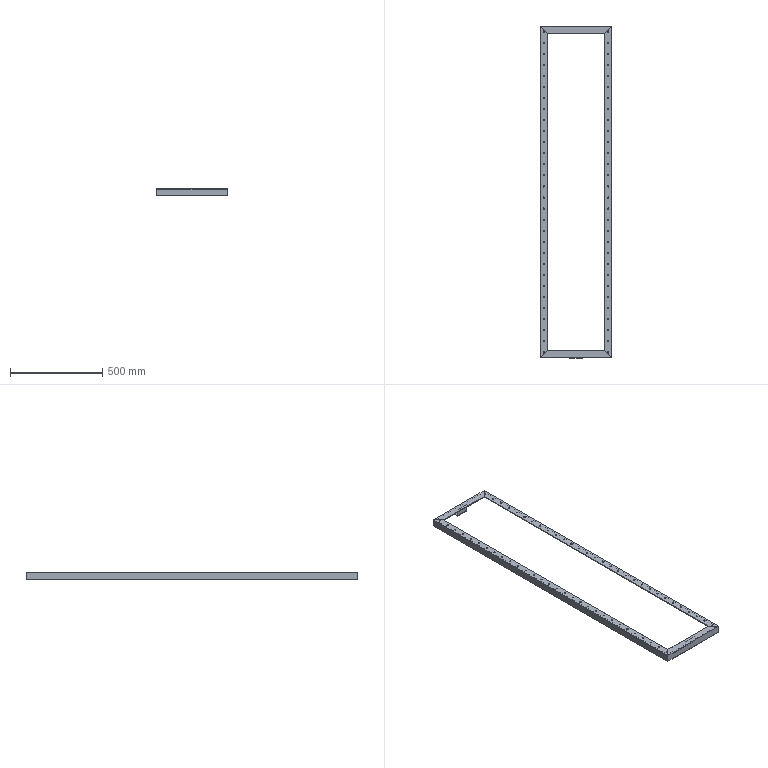Part | SolidWorks | features ICE 2, WeldMemberFeat 1, WeldmentFeature 1 | 6 solids | 180 faces | box 390 x 1800 x 43 mm | volume 1342182 mm3 | cylinder 132 | plane 48 | commonest cylinder face diameters 6.5 x120 2.667 x8 10 x4